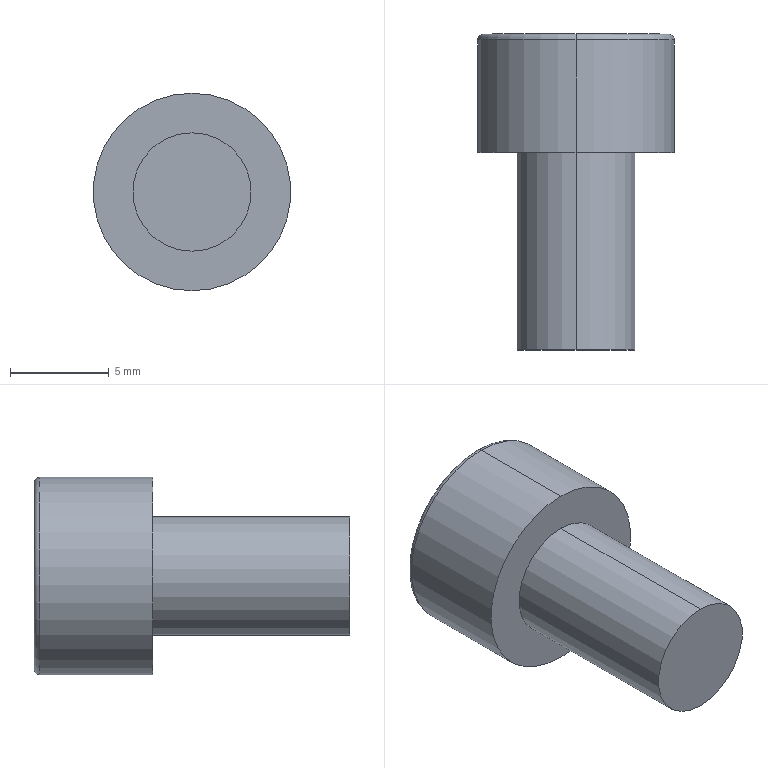Part | STEP file | M6 socket head cap screw simplified_M6X10 | 1 solid | 16 faces | box 10 x 16 x 10 mm | volume 685.808 mm3 | plane 10 | cylinder 4 | torus 2 | commonest cylinder face diameters 6 x2 10 x2
STEP:
#1=CARTESIAN_POINT('',(0.,0.,0.));
#2=DIRECTION('',(0.,0.,1.));
#3=DIRECTION('',(1.,0.,0.));
#4=AXIS2_PLACEMENT_3D('',#1,#2,#3);
#5=CARTESIAN_POINT('',(0.,0.,4.7));
#6=VERTEX_POINT('',#5);
#7=CARTESIAN_POINT('',(0.,0.,-4.7));
#8=VERTEX_POINT('',#7);
#9=CARTESIAN_POINT('',(0.,0.,0.));
#10=DIRECTION('',(0.,1.,0.));
#11=DIRECTION('',(0.,0.,-1.));
#12=AXIS2_PLACEMENT_3D('',#9,#10,#11);
#13=CIRCLE('',#12,4.7);
#14=CARTESIAN_POINT('',(0.,-0.3,0.));
#15=DIRECTION('',(0.,-1.,0.));
#16=DIRECTION('',(0.,0.,-1.));
#17=AXIS2_PLACEMENT_3D('',#14,#15,#16);
#18=TOROIDAL_SURFACE('',#17,4.7,0.3);
#19=CARTESIAN_POINT('',(6.283,4.712));
#20=DIRECTION('',(-1.,0.));
#21=VECTOR('',#20,1.);
#22=LINE('',#19,#21);
#23=(GEOMETRIC_REPRESENTATION_CONTEXT(2)PARAMETRIC_REPRESENTATION_CONTEXT()REPRESENTATION_CONTEXT('',''));
#24=DEFINITIONAL_REPRESENTATION('',(#22),#23);
#25=PCURVE('',#18,#24);
#26=CARTESIAN_POINT('',(0.,0.,0.));
#27=DIRECTION('',(0.,-1.,0.));
#28=DIRECTION('',(0.,0.,-1.));
#29=AXIS2_PLACEMENT_3D('',#26,#27,#28);
#30=PLANE('',#29);
#31=CARTESIAN_POINT('',(4.7,0.));
#32=CARTESIAN_POINT('',(4.7,-8.141));
#33=CARTESIAN_POINT('',(-2.35,-4.07));
#34=CARTESIAN_POINT('',(-9.4,0.));
#35=CARTESIAN_POINT('',(-2.35,4.07));
#36=CARTESIAN_POINT('',(4.7,8.141));
#37=CARTESIAN_POINT('',(4.7,0.));
#38=(BOUNDED_CURVE()B_SPLINE_CURVE(2,(#31,#32,#33,#34,#35,#36,#37),.UNSPECIFIED.,.T.,.F.)B_SPLINE_CURVE_WITH_KNOTS((1,2,2,2,2,1),(-2.094,0.,2.094,4.189,6.283,8.378),.UNSPECIFIED.)CURVE()GEOMETRIC_REPRESENTATION_ITEM()RATIONAL_B_SPLINE_CURVE((1.,0.5,1.,0.5,1.,0.5,1.))REPRESENTATION_ITEM(''));
#39=(GEOMETRIC_REPRESENTATION_CONTEXT(2)PARAMETRIC_REPRESENTATION_CONTEXT()REPRESENTATION_CONTEXT('',''));
#40=DEFINITIONAL_REPRESENTATION('',(#38),#39);
#41=PCURVE('',#30,#40);
#42=SURFACE_CURVE('',#13,(#25,#41),.PCURVE_S1.);
#43=EDGE_CURVE('',#6,#8,#42,.T.);
#44=ORIENTED_EDGE('',*,*,#43,.F.);
#45=CARTESIAN_POINT('',(0.,-0.3,5.));
#46=VERTEX_POINT('',#45);
#47=CARTESIAN_POINT('',(0.,-0.3,4.7));
#48=DIRECTION('',(1.,0.,0.));
#49=DIRECTION('',(0.,0.,-1.));
#50=AXIS2_PLACEMENT_3D('',#47,#48,#49);
#51=CIRCLE('',#50,0.3);
#52=CARTESIAN_POINT('',(3.142,3.142));
#53=DIRECTION('',(0.,1.));
#54=VECTOR('',#53,1.);
#55=LINE('',#52,#54);
#56=(GEOMETRIC_REPRESENTATION_CONTEXT(2)PARAMETRIC_REPRESENTATION_CONTEXT()REPRESENTATION_CONTEXT('',''));
#57=DEFINITIONAL_REPRESENTATION('',(#55),#56);
#58=PCURVE('',#18,#57);
#59=CARTESIAN_POINT('',(0.,-0.3,0.));
#60=DIRECTION('',(0.,-1.,0.));
#61=DIRECTION('',(0.,0.,-1.));
#62=AXIS2_PLACEMENT_3D('',#59,#60,#61);
#63=TOROIDAL_SURFACE('',#62,4.7,0.3);
#64=CARTESIAN_POINT('',(3.142,3.142));
#65=DIRECTION('',(0.,1.));
#66=VECTOR('',#65,1.);
#67=LINE('',#64,#66);
#68=(GEOMETRIC_REPRESENTATION_CONTEXT(2)PARAMETRIC_REPRESENTATION_CONTEXT()REPRESENTATION_CONTEXT('',''));
#69=DEFINITIONAL_REPRESENTATION('',(#67),#68);
#70=PCURVE('',#63,#69);
#71=SURFACE_CURVE('',#51,(#58,#70),.PCURVE_S1.);
#72=EDGE_CURVE('',#6,#46,#71,.T.);
#73=ORIENTED_EDGE('',*,*,#72,.T.);
#74=CARTESIAN_POINT('',(0.,-0.3,-5.));
#75=VERTEX_POINT('',#74);
#76=CARTESIAN_POINT('',(0.,-0.3,0.));
#77=DIRECTION('',(0.,-1.,0.));
#78=DIRECTION('',(0.,0.,-1.));
#79=AXIS2_PLACEMENT_3D('',#76,#77,#78);
#80=CIRCLE('',#79,5.);
#81=CARTESIAN_POINT('',(0.,6.283));
#82=DIRECTION('',(1.,0.));
#83=VECTOR('',#82,1.);
#84=LINE('',#81,#83);
#85=(GEOMETRIC_REPRESENTATION_CONTEXT(2)PARAMETRIC_REPRESENTATION_CONTEXT()REPRESENTATION_CONTEXT('',''));
#86=DEFINITIONAL_REPRESENTATION('',(#84),#85);
#87=PCURVE('',#18,#86);
#88=CARTESIAN_POINT('',(0.,0.,0.));
#89=DIRECTION('',(0.,1.,0.));
#90=DIRECTION('',(0.,0.,1.));
#91=AXIS2_PLACEMENT_3D('',#88,#89,#90);
#92=CYLINDRICAL_SURFACE('',#91,5.);
#93=CARTESIAN_POINT('',(3.142,-0.3));
#94=DIRECTION('',(-1.,0.));
#95=VECTOR('',#94,1.);
#96=LINE('',#93,#95);
#97=(GEOMETRIC_REPRESENTATION_CONTEXT(2)PARAMETRIC_REPRESENTATION_CONTEXT()REPRESENTATION_CONTEXT('',''));
#98=DEFINITIONAL_REPRESENTATION('',(#96),#97);
#99=PCURVE('',#92,#98);
#100=SURFACE_CURVE('',#80,(#87,#99),.PCURVE_S1.);
#101=EDGE_CURVE('',#75,#46,#100,.T.);
#102=ORIENTED_EDGE('',*,*,#101,.F.);
#103=CARTESIAN_POINT('',(0.,-0.3,-4.7));
#104=DIRECTION('',(-1.,0.,0.));
#105=DIRECTION('',(0.,0.,1.));
#106=AXIS2_PLACEMENT_3D('',#103,#104,#105);
#107=CIRCLE('',#106,0.3);
#108=CARTESIAN_POINT('',(0.,3.142));
#109=DIRECTION('',(0.,1.));
#110=VECTOR('',#109,1.);
#111=LINE('',#108,#110);
#112=(GEOMETRIC_REPRESENTATION_CONTEXT(2)PARAMETRIC_REPRESENTATION_CONTEXT()REPRESENTATION_CONTEXT('',''));
#113=DEFINITIONAL_REPRESENTATION('',(#111),#112);
#114=PCURVE('',#18,#113);
#115=CARTESIAN_POINT('',(6.283,3.142));
#116=DIRECTION('',(0.,1.));
#117=VECTOR('',#116,1.);
#118=LINE('',#115,#117);
#119=(GEOMETRIC_REPRESENTATION_CONTEXT(2)PARAMETRIC_REPRESENTATION_CONTEXT()REPRESENTATION_CONTEXT('',''));
#120=DEFINITIONAL_REPRESENTATION('',(#118),#119);
#121=PCURVE('',#63,#120);
#122=SURFACE_CURVE('',#107,(#114,#121),.PCURVE_S1.);
#123=EDGE_CURVE('',#8,#75,#122,.T.);
#124=ORIENTED_EDGE('',*,*,#123,.F.);
#125=EDGE_LOOP('',(#44,#73,#102,#124));
#126=FACE_BOUND('',#125,.T.);
#127=ADVANCED_FACE('',(#126),#18,.T.);
#128=CARTESIAN_POINT('',(0.,-16.,3.));
#129=VERTEX_POINT('',#128);
#130=CARTESIAN_POINT('',(0.,-16.,-3.));
#131=VERTEX_POINT('',#130);
#132=CARTESIAN_POINT('',(0.,-16.,0.));
#133=DIRECTION('',(0.,1.,0.));
#134=DIRECTION('',(0.,0.,1.));
#135=AXIS2_PLACEMENT_3D('',#132,#133,#134);
#136=CIRCLE('',#135,3.);
#137=CARTESIAN_POINT('',(0.,0.,0.));
#138=DIRECTION('',(0.,1.,0.));
#139=DIRECTION('',(0.,0.,1.));
#140=AXIS2_PLACEMENT_3D('',#137,#138,#139);
#141=CYLINDRICAL_SURFACE('',#140,3.);
#142=CARTESIAN_POINT('',(0.,-16.));
#143=DIRECTION('',(1.,0.));
#144=VECTOR('',#143,1.);
#145=LINE('',#142,#144);
#146=(GEOMETRIC_REPRESENTATION_CONTEXT(2)PARAMETRIC_REPRESENTATION_CONTEXT()REPRESENTATION_CONTEXT('',''));
#147=DEFINITIONAL_REPRESENTATION('',(#145),#146);
#148=PCURVE('',#141,#147);
#149=CARTESIAN_POINT('',(3.,-16.,0.));
#150=DIRECTION('',(0.,1.,0.));
#151=DIRECTION('',(0.,0.,1.));
#152=AXIS2_PLACEMENT_3D('',#149,#150,#151);
#153=PLANE('',#152);
#154=CARTESIAN_POINT('',(0.,-3.));
#155=DIRECTION('',(1.,0.));
#156=AXIS2_PLACEMENT_2D('',#154,#155);
#157=CIRCLE('',#156,3.);
#158=(GEOMETRIC_REPRESENTATION_CONTEXT(2)PARAMETRIC_REPRESENTATION_CONTEXT()REPRESENTATION_CONTEXT('',''));
#159=DEFINITIONAL_REPRESENTATION('',(#157),#158);
#160=PCURVE('',#153,#159);
#161=SURFACE_CURVE('',#136,(#148,#160),.PCURVE_S1.);
#162=EDGE_CURVE('',#129,#131,#161,.T.);
#163=ORIENTED_EDGE('',*,*,#162,.T.);
#164=CARTESIAN_POINT('',(0.,-6.,-3.));
#165=VERTEX_POINT('',#164);
#166=CARTESIAN_POINT('',(0.,0.,-3.));
#167=DIRECTION('',(0.,1.,0.));
#168=VECTOR('',#167,1.);
#169=LINE('',#166,#168);
#170=CARTESIAN_POINT('',(3.142,0.));
#171=DIRECTION('',(0.,1.));
#172=VECTOR('',#171,1.);
#173=LINE('',#170,#172);
#174=(GEOMETRIC_REPRESENTATION_CONTEXT(2)PARAMETRIC_REPRESENTATION_CONTEXT()REPRESENTATION_CONTEXT('',''));
#175=DEFINITIONAL_REPRESENTATION('',(#173),#174);
#176=PCURVE('',#141,#175);
#177=CARTESIAN_POINT('',(0.,0.,0.));
#178=DIRECTION('',(0.,1.,0.));
#179=DIRECTION('',(0.,0.,1.));
#180=AXIS2_PLACEMENT_3D('',#177,#178,#179);
#181=CYLINDRICAL_SURFACE('',#180,3.);
#182=CARTESIAN_POINT('',(3.142,0.));
#183=DIRECTION('',(0.,1.));
#184=VECTOR('',#183,1.);
#185=LINE('',#182,#184);
#186=(GEOMETRIC_REPRESENTATION_CONTEXT(2)PARAMETRIC_REPRESENTATION_CONTEXT()REPRESENTATION_CONTEXT('',''));
#187=DEFINITIONAL_REPRESENTATION('',(#185),#186);
#188=PCURVE('',#181,#187);
#189=SURFACE_CURVE('',#169,(#176,#188),.PCURVE_S1.);
#190=EDGE_CURVE('',#131,#165,#189,.T.);
#191=ORIENTED_EDGE('',*,*,#190,.T.);
#192=CARTESIAN_POINT('',(0.,-6.,3.));
#193=VERTEX_POINT('',#192);
#194=CARTESIAN_POINT('',(0.,-6.,0.));
#195=DIRECTION('',(0.,1.,0.));
#196=DIRECTION('',(0.,0.,1.));
#197=AXIS2_PLACEMENT_3D('',#194,#195,#196);
#198=CIRCLE('',#197,3.);
#199=CARTESIAN_POINT('',(0.,-6.));
#200=DIRECTION('',(1.,0.));
#201=VECTOR('',#200,1.);
#202=LINE('',#199,#201);
#203=(GEOMETRIC_REPRESENTATION_CONTEXT(2)PARAMETRIC_REPRESENTATION_CONTEXT()REPRESENTATION_CONTEXT('',''));
#204=DEFINITIONAL_REPRESENTATION('',(#202),#203);
#205=PCURVE('',#141,#204);
#206=CARTESIAN_POINT('',(5.,-6.,0.));
#207=DIRECTION('',(0.,1.,0.));
#208=DIRECTION('',(0.,0.,1.));
#209=AXIS2_PLACEMENT_3D('',#206,#207,#208);
#210=PLANE('',#209);
#211=CARTESIAN_POINT('',(0.,-5.));
#212=DIRECTION('',(1.,0.));
#213=AXIS2_PLACEMENT_2D('',#211,#212);
#214=CIRCLE('',#213,3.);
#215=(GEOMETRIC_REPRESENTATION_CONTEXT(2)PARAMETRIC_REPRESENTATION_CONTEXT()REPRESENTATION_CONTEXT('',''));
#216=DEFINITIONAL_REPRESENTATION('',(#214),#215);
#217=PCURVE('',#210,#216);
#218=SURFACE_CURVE('',#198,(#205,#217),.PCURVE_S1.);
#219=EDGE_CURVE('',#193,#165,#218,.T.);
#220=ORIENTED_EDGE('',*,*,#219,.F.);
#221=CARTESIAN_POINT('',(0.,0.,3.));
#222=DIRECTION('',(0.,1.,0.));
#223=VECTOR('',#222,1.);
#224=LINE('',#221,#223);
#225=CARTESIAN_POINT('',(0.,0.));
#226=DIRECTION('',(0.,1.));
#227=VECTOR('',#226,1.);
#228=LINE('',#225,#227);
#229=(GEOMETRIC_REPRESENTATION_CONTEXT(2)PARAMETRIC_REPRESENTATION_CONTEXT()REPRESENTATION_CONTEXT('',''));
#230=DEFINITIONAL_REPRESENTATION('',(#228),#229);
#231=PCURVE('',#141,#230);
#232=CARTESIAN_POINT('',(6.283,0.));
#233=DIRECTION('',(0.,1.));
#234=VECTOR('',#233,1.);
#235=LINE('',#232,#234);
#236=(GEOMETRIC_REPRESENTATION_CONTEXT(2)PARAMETRIC_REPRESENTATION_CONTEXT()REPRESENTATION_CONTEXT('',''));
#237=DEFINITIONAL_REPRESENTATION('',(#235),#236);
#238=PCURVE('',#181,#237);
#239=SURFACE_CURVE('',#224,(#231,#238),.PCURVE_S1.);
#240=EDGE_CURVE('',#129,#193,#239,.T.);
#241=ORIENTED_EDGE('',*,*,#240,.F.);
#242=EDGE_LOOP('',(#163,#191,#220,#241));
#243=FACE_BOUND('',#242,.T.);
#244=ADVANCED_FACE('',(#243),#141,.T.);
#245=CARTESIAN_POINT('',(0.,-6.,5.));
#246=VERTEX_POINT('',#245);
#247=CARTESIAN_POINT('',(0.,-6.,-5.));
#248=VERTEX_POINT('',#247);
#249=CARTESIAN_POINT('',(0.,-6.,0.));
#250=DIRECTION('',(0.,1.,0.));
#251=DIRECTION('',(0.,0.,1.));
#252=AXIS2_PLACEMENT_3D('',#249,#250,#251);
#253=CIRCLE('',#252,5.);
#254=CARTESIAN_POINT('',(0.,-6.));
#255=DIRECTION('',(1.,0.));
#256=VECTOR('',#255,1.);
#257=LINE('',#254,#256);
#258=(GEOMETRIC_REPRESENTATION_CONTEXT(2)PARAMETRIC_REPRESENTATION_CONTEXT()REPRESENTATION_CONTEXT('',''));
#259=DEFINITIONAL_REPRESENTATION('',(#257),#258);
#260=PCURVE('',#92,#259);
#261=CARTESIAN_POINT('',(0.,-5.));
#262=DIRECTION('',(1.,0.));
#263=AXIS2_PLACEMENT_2D('',#261,#262);
#264=CIRCLE('',#263,5.);
#265=(GEOMETRIC_REPRESENTATION_CONTEXT(2)PARAMETRIC_REPRESENTATION_CONTEXT()REPRESENTATION_CONTEXT('',''));
#266=DEFINITIONAL_REPRESENTATION('',(#264),#265);
#267=PCURVE('',#210,#266);
#268=SURFACE_CURVE('',#253,(#260,#267),.PCURVE_S1.);
#269=EDGE_CURVE('',#246,#248,#268,.T.);
#270=ORIENTED_EDGE('',*,*,#269,.T.);
#271=CARTESIAN_POINT('',(0.,0.,-5.));
#272=DIRECTION('',(0.,1.,0.));
#273=VECTOR('',#272,1.);
#274=LINE('',#271,#273);
#275=CARTESIAN_POINT('',(3.142,0.));
#276=DIRECTION('',(0.,1.));
#277=VECTOR('',#276,1.);
#278=LINE('',#275,#277);
#279=(GEOMETRIC_REPRESENTATION_CONTEXT(2)PARAMETRIC_REPRESENTATION_CONTEXT()REPRESENTATION_CONTEXT('',''));
#280=DEFINITIONAL_REPRESENTATION('',(#278),#279);
#281=PCURVE('',#92,#280);
#282=CARTESIAN_POINT('',(0.,0.,0.));
#283=DIRECTION('',(0.,1.,0.));
#284=DIRECTION('',(0.,0.,1.));
#285=AXIS2_PLACEMENT_3D('',#282,#283,#284);
#286=CYLINDRICAL_SURFACE('',#285,5.);
#287=CARTESIAN_POINT('',(3.142,0.));
#288=DIRECTION('',(0.,1.));
#289=VECTOR('',#288,1.);
#290=LINE('',#287,#289);
#291=(GEOMETRIC_REPRESENTATION_CONTEXT(2)PARAMETRIC_REPRESENTATION_CONTEXT()REPRESENTATION_CONTEXT('',''));
#292=DEFINITIONAL_REPRESENTATION('',(#290),#291);
#293=PCURVE('',#286,#292);
#294=SURFACE_CURVE('',#274,(#281,#293),.PCURVE_S1.);
#295=EDGE_CURVE('',#248,#75,#294,.T.);
#296=ORIENTED_EDGE('',*,*,#295,.T.);
#297=ORIENTED_EDGE('',*,*,#101,.T.);
#298=CARTESIAN_POINT('',(0.,0.,5.));
#299=DIRECTION('',(0.,1.,0.));
#300=VECTOR('',#299,1.);
#301=LINE('',#298,#300);
#302=CARTESIAN_POINT('',(0.,0.));
#303=DIRECTION('',(0.,1.));
#304=VECTOR('',#303,1.);
#305=LINE('',#302,#304);
#306=(GEOMETRIC_REPRESENTATION_CONTEXT(2)PARAMETRIC_REPRESENTATION_CONTEXT()REPRESENTATION_CONTEXT('',''));
#307=DEFINITIONAL_REPRESENTATION('',(#305),#306);
#308=PCURVE('',#92,#307);
#309=CARTESIAN_POINT('',(6.283,0.));
#310=DIRECTION('',(0.,1.));
#311=VECTOR('',#310,1.);
#312=LINE('',#309,#311);
#313=(GEOMETRIC_REPRESENTATION_CONTEXT(2)PARAMETRIC_REPRESENTATION_CONTEXT()REPRESENTATION_CONTEXT('',''));
#314=DEFINITIONAL_REPRESENTATION('',(#312),#313);
#315=PCURVE('',#286,#314);
#316=SURFACE_CURVE('',#301,(#308,#315),.PCURVE_S1.);
#317=EDGE_CURVE('',#246,#46,#316,.T.);
#318=ORIENTED_EDGE('',*,*,#317,.F.);
#319=EDGE_LOOP('',(#270,#296,#297,#318));
#320=FACE_BOUND('',#319,.T.);
#321=ADVANCED_FACE('',(#320),#92,.T.);
#322=CARTESIAN_POINT('',(0.,0.,0.));
#323=DIRECTION('',(0.,1.,0.));
#324=DIRECTION('',(0.,0.,-1.));
#325=AXIS2_PLACEMENT_3D('',#322,#323,#324);
#326=CIRCLE('',#325,4.7);
#327=CARTESIAN_POINT('',(4.7,0.));
#328=CARTESIAN_POINT('',(4.7,-8.141));
#329=CARTESIAN_POINT('',(-2.35,-4.07));
#330=CARTESIAN_POINT('',(-9.4,0.));
#331=CARTESIAN_POINT('',(-2.35,4.07));
#332=CARTESIAN_POINT('',(4.7,8.141));
#333=CARTESIAN_POINT('',(4.7,0.));
#334=(BOUNDED_CURVE()B_SPLINE_CURVE(2,(#327,#328,#329,#330,#331,#332,#333),.UNSPECIFIED.,.T.,.F.)B_SPLINE_CURVE_WITH_KNOTS((1,2,2,2,2,1),(-2.094,0.,2.094,4.189,6.283,8.378),.UNSPECIFIED.)CURVE()GEOMETRIC_REPRESENTATION_ITEM()RATIONAL_B_SPLINE_CURVE((1.,0.5,1.,0.5,1.,0.5,1.))REPRESENTATION_ITEM(''));
#335=(GEOMETRIC_REPRESENTATION_CONTEXT(2)PARAMETRIC_REPRESENTATION_CONTEXT()REPRESENTATION_CONTEXT('',''));
#336=DEFINITIONAL_REPRESENTATION('',(#334),#335);
#337=PCURVE('',#30,#336);
#338=CARTESIAN_POINT('',(6.283,4.712));
#339=DIRECTION('',(-1.,0.));
#340=VECTOR('',#339,1.);
#341=LINE('',#338,#340);
#342=(GEOMETRIC_REPRESENTATION_CONTEXT(2)PARAMETRIC_REPRESENTATION_CONTEXT()REPRESENTATION_CONTEXT('',''));
#343=DEFINITIONAL_REPRESENTATION('',(#341),#342);
#344=PCURVE('',#63,#343);
#345=SURFACE_CURVE('',#326,(#337,#344),.PCURVE_S1.);
#346=EDGE_CURVE('',#8,#6,#345,.T.);
#347=ORIENTED_EDGE('',*,*,#346,.T.);
#348=ORIENTED_EDGE('',*,*,#43,.T.);
#349=EDGE_LOOP('',(#347,#348));
#350=FACE_BOUND('',#349,.T.);
#351=CARTESIAN_POINT('',(-2.944,0.,0.));
#352=VERTEX_POINT('',#351);
#353=CARTESIAN_POINT('',(-1.472,0.,2.55));
#354=VERTEX_POINT('',#353);
#355=CARTESIAN_POINT('',(-2.944,0.,0.));
#356=DIRECTION('',(0.5,0.,0.866));
#357=VECTOR('',#356,1.);
#358=LINE('',#355,#357);
#359=CARTESIAN_POINT('',(0.,-2.944));
#360=DIRECTION('',(-0.866,0.5));
#361=VECTOR('',#360,1.);
#362=LINE('',#359,#361);
#363=(GEOMETRIC_REPRESENTATION_CONTEXT(2)PARAMETRIC_REPRESENTATION_CONTEXT()REPRESENTATION_CONTEXT('',''));
#364=DEFINITIONAL_REPRESENTATION('',(#362),#363);
#365=PCURVE('',#30,#364);
#366=CARTESIAN_POINT('',(-2.944,-3.,0.));
#367=DIRECTION('',(-0.866,0.,0.5));
#368=DIRECTION('',(0.5,0.,0.866));
#369=AXIS2_PLACEMENT_3D('',#366,#367,#368);
#370=PLANE('',#369);
#371=CARTESIAN_POINT('',(0.,3.));
#372=DIRECTION('',(1.,0.));
#373=VECTOR('',#372,1.);
#374=LINE('',#371,#373);
#375=(GEOMETRIC_REPRESENTATION_CONTEXT(2)PARAMETRIC_REPRESENTATION_CONTEXT()REPRESENTATION_CONTEXT('',''));
#376=DEFINITIONAL_REPRESENTATION('',(#374),#375);
#377=PCURVE('',#370,#376);
#378=SURFACE_CURVE('',#358,(#365,#377),.PCURVE_S1.);
#379=EDGE_CURVE('',#352,#354,#378,.T.);
#380=ORIENTED_EDGE('',*,*,#379,.F.);
#381=CARTESIAN_POINT('',(-1.472,0.,-2.55));
#382=VERTEX_POINT('',#381);
#383=CARTESIAN_POINT('',(-1.472,0.,-2.55));
#384=DIRECTION('',(-0.5,0.,0.866));
#385=VECTOR('',#384,1.);
#386=LINE('',#383,#385);
#387=CARTESIAN_POINT('',(2.55,-1.472));
#388=DIRECTION('',(-0.866,-0.5));
#389=VECTOR('',#388,1.);
#390=LINE('',#387,#389);
#391=(GEOMETRIC_REPRESENTATION_CONTEXT(2)PARAMETRIC_REPRESENTATION_CONTEXT()REPRESENTATION_CONTEXT('',''));
#392=DEFINITIONAL_REPRESENTATION('',(#390),#391);
#393=PCURVE('',#30,#392);
#394=CARTESIAN_POINT('',(-1.472,-3.,-2.55));
#395=DIRECTION('',(-0.866,0.,-0.5));
#396=DIRECTION('',(-0.5,0.,0.866));
#397=AXIS2_PLACEMENT_3D('',#394,#395,#396);
#398=PLANE('',#397);
#399=CARTESIAN_POINT('',(0.,3.));
#400=DIRECTION('',(1.,0.));
#401=VECTOR('',#400,1.);
#402=LINE('',#399,#401);
#403=(GEOMETRIC_REPRESENTATION_CONTEXT(2)PARAMETRIC_REPRESENTATION_CONTEXT()REPRESENTATION_CONTEXT('',''));
#404=DEFINITIONAL_REPRESENTATION('',(#402),#403);
#405=PCURVE('',#398,#404);
#406=SURFACE_CURVE('',#386,(#393,#405),.PCURVE_S1.);
#407=EDGE_CURVE('',#382,#352,#406,.T.);
#408=ORIENTED_EDGE('',*,*,#407,.F.);
#409=CARTESIAN_POINT('',(1.472,0.,-2.55));
#410=VERTEX_POINT('',#409);
#411=CARTESIAN_POINT('',(1.472,0.,-2.55));
#412=DIRECTION('',(-1.,0.,0.));
#413=VECTOR('',#412,1.);
#414=LINE('',#411,#413);
#415=CARTESIAN_POINT('',(2.55,1.472));
#416=DIRECTION('',(0.,-1.));
#417=VECTOR('',#416,1.);
#418=LINE('',#415,#417);
#419=(GEOMETRIC_REPRESENTATION_CONTEXT(2)PARAMETRIC_REPRESENTATION_CONTEXT()REPRESENTATION_CONTEXT('',''));
#420=DEFINITIONAL_REPRESENTATION('',(#418),#419);
#421=PCURVE('',#30,#420);
#422=CARTESIAN_POINT('',(1.472,-3.,-2.55));
#423=DIRECTION('',(0.,0.,-1.));
#424=DIRECTION('',(-1.,0.,0.));
#425=AXIS2_PLACEMENT_3D('',#422,#423,#424);
#426=PLANE('',#425);
#427=CARTESIAN_POINT('',(0.,3.));
#428=DIRECTION('',(1.,0.));
#429=VECTOR('',#428,1.);
#430=LINE('',#427,#429);
#431=(GEOMETRIC_REPRESENTATION_CONTEXT(2)PARAMETRIC_REPRESENTATION_CONTEXT()REPRESENTATION_CONTEXT('',''));
#432=DEFINITIONAL_REPRESENTATION('',(#430),#431);
#433=PCURVE('',#426,#432);
#434=SURFACE_CURVE('',#414,(#421,#433),.PCURVE_S1.);
#435=EDGE_CURVE('',#410,#382,#434,.T.);
#436=ORIENTED_EDGE('',*,*,#435,.F.);
#437=CARTESIAN_POINT('',(2.944,0.,0.));
#438=VERTEX_POINT('',#437);
#439=CARTESIAN_POINT('',(2.944,0.,0.));
#440=DIRECTION('',(-0.5,0.,-0.866));
#441=VECTOR('',#440,1.);
#442=LINE('',#439,#441);
#443=CARTESIAN_POINT('',(0.,2.944));
#444=DIRECTION('',(0.866,-0.5));
#445=VECTOR('',#444,1.);
#446=LINE('',#443,#445);
#447=(GEOMETRIC_REPRESENTATION_CONTEXT(2)PARAMETRIC_REPRESENTATION_CONTEXT()REPRESENTATION_CONTEXT('',''));
#448=DEFINITIONAL_REPRESENTATION('',(#446),#447);
#449=PCURVE('',#30,#448);
#450=CARTESIAN_POINT('',(2.944,-3.,0.));
#451=DIRECTION('',(0.866,0.,-0.5));
#452=DIRECTION('',(-0.5,0.,-0.866));
#453=AXIS2_PLACEMENT_3D('',#450,#451,#452);
#454=PLANE('',#453);
#455=CARTESIAN_POINT('',(0.,3.));
#456=DIRECTION('',(1.,0.));
#457=VECTOR('',#456,1.);
#458=LINE('',#455,#457);
#459=(GEOMETRIC_REPRESENTATION_CONTEXT(2)PARAMETRIC_REPRESENTATION_CONTEXT()REPRESENTATION_CONTEXT('',''));
#460=DEFINITIONAL_REPRESENTATION('',(#458),#459);
#461=PCURVE('',#454,#460);
#462=SURFACE_CURVE('',#442,(#449,#461),.PCURVE_S1.);
#463=EDGE_CURVE('',#438,#410,#462,.T.);
#464=ORIENTED_EDGE('',*,*,#463,.F.);
#465=CARTESIAN_POINT('',(1.472,0.,2.55));
#466=VERTEX_POINT('',#465);
#467=CARTESIAN_POINT('',(1.472,0.,2.55));
#468=DIRECTION('',(0.5,0.,-0.866));
#469=VECTOR('',#468,1.);
#470=LINE('',#467,#469);
#471=CARTESIAN_POINT('',(-2.55,1.472));
#472=DIRECTION('',(0.866,0.5));
#473=VECTOR('',#472,1.);
#474=LINE('',#471,#473);
#475=(GEOMETRIC_REPRESENTATION_CONTEXT(2)PARAMETRIC_REPRESENTATION_CONTEXT()REPRESENTATION_CONTEXT('',''));
#476=DEFINITIONAL_REPRESENTATION('',(#474),#475);
#477=PCURVE('',#30,#476);
#478=CARTESIAN_POINT('',(1.472,-3.,2.55));
#479=DIRECTION('',(0.866,0.,0.5));
#480=DIRECTION('',(0.5,0.,-0.866));
#481=AXIS2_PLACEMENT_3D('',#478,#479,#480);
#482=PLANE('',#481);
#483=CARTESIAN_POINT('',(0.,3.));
#484=DIRECTION('',(1.,0.));
#485=VECTOR('',#484,1.);
#486=LINE('',#483,#485);
#487=(GEOMETRIC_REPRESENTATION_CONTEXT(2)PARAMETRIC_REPRESENTATION_CONTEXT()REPRESENTATION_CONTEXT('',''));
#488=DEFINITIONAL_REPRESENTATION('',(#486),#487);
#489=PCURVE('',#482,#488);
#490=SURFACE_CURVE('',#470,(#477,#489),.PCURVE_S1.);
#491=EDGE_CURVE('',#466,#438,#490,.T.);
#492=ORIENTED_EDGE('',*,*,#491,.F.);
#493=CARTESIAN_POINT('',(-1.472,0.,2.55));
#494=DIRECTION('',(1.,0.,0.));
#495=VECTOR('',#494,1.);
#496=LINE('',#493,#495);
#497=CARTESIAN_POINT('',(-2.55,-1.472));
#498=DIRECTION('',(0.,1.));
#499=VECTOR('',#498,1.);
#500=LINE('',#497,#499);
#501=(GEOMETRIC_REPRESENTATION_CONTEXT(2)PARAMETRIC_REPRESENTATION_CONTEXT()REPRESENTATION_CONTEXT('',''));
#502=DEFINITIONAL_REPRESENTATION('',(#500),#501);
#503=PCURVE('',#30,#502);
#504=CARTESIAN_POINT('',(-1.472,-3.,2.55));
#505=DIRECTION('',(0.,0.,1.));
#506=DIRECTION('',(1.,0.,0.));
#507=AXIS2_PLACEMENT_3D('',#504,#505,#506);
#508=PLANE('',#507);
#509=CARTESIAN_POINT('',(0.,3.));
#510=DIRECTION('',(1.,0.));
#511=VECTOR('',#510,1.);
#512=LINE('',#509,#511);
#513=(GEOMETRIC_REPRESENTATION_CONTEXT(2)PARAMETRIC_REPRESENTATION_CONTEXT()REPRESENTATION_CONTEXT('',''));
#514=DEFINITIONAL_REPRESENTATION('',(#512),#513);
#515=PCURVE('',#508,#514);
#516=SURFACE_CURVE('',#496,(#503,#515),.PCURVE_S1.);
#517=EDGE_CURVE('',#354,#466,#516,.T.);
#518=ORIENTED_EDGE('',*,*,#517,.F.);
#519=EDGE_LOOP('',(#380,#408,#436,#464,#492,#518));
#520=FACE_BOUND('',#519,.T.);
#521=ADVANCED_FACE('',(#350,#520),#30,.F.);
#522=ORIENTED_EDGE('',*,*,#295,.F.);
#523=CARTESIAN_POINT('',(0.,-6.,0.));
#524=DIRECTION('',(0.,1.,0.));
#525=DIRECTION('',(0.,0.,1.));
#526=AXIS2_PLACEMENT_3D('',#523,#524,#525);
#527=CIRCLE('',#526,5.);
#528=CARTESIAN_POINT('',(0.,-6.));
#529=DIRECTION('',(1.,0.));
#530=VECTOR('',#529,1.);
#531=LINE('',#528,#530);
#532=(GEOMETRIC_REPRESENTATION_CONTEXT(2)PARAMETRIC_REPRESENTATION_CONTEXT()REPRESENTATION_CONTEXT('',''));
#533=DEFINITIONAL_REPRESENTATION('',(#531),#532);
#534=PCURVE('',#286,#533);
#535=CARTESIAN_POINT('',(0.,-5.));
#536=DIRECTION('',(1.,0.));
#537=AXIS2_PLACEMENT_2D('',#535,#536);
#538=CIRCLE('',#537,5.);
#539=(GEOMETRIC_REPRESENTATION_CONTEXT(2)PARAMETRIC_REPRESENTATION_CONTEXT()REPRESENTATION_CONTEXT('',''));
#540=DEFINITIONAL_REPRESENTATION('',(#538),#539);
#541=PCURVE('',#210,#540);
#542=SURFACE_CURVE('',#527,(#534,#541),.PCURVE_S1.);
#543=EDGE_CURVE('',#248,#246,#542,.T.);
#544=ORIENTED_EDGE('',*,*,#543,.T.);
#545=ORIENTED_EDGE('',*,*,#317,.T.);
#546=CARTESIAN_POINT('',(0.,-0.3,0.));
#547=DIRECTION('',(0.,-1.,0.));
#548=DIRECTION('',(0.,0.,-1.));
#549=AXIS2_PLACEMENT_3D('',#546,#547,#548);
#550=CIRCLE('',#549,5.);
#551=CARTESIAN_POINT('',(9.425,-0.3));
#552=DIRECTION('',(-1.,0.));
#553=VECTOR('',#552,1.);
#554=LINE('',#551,#553);
#555=(GEOMETRIC_REPRESENTATION_CONTEXT(2)PARAMETRIC_REPRESENTATION_CONTEXT()REPRESENTATION_CONTEXT('',''));
#556=DEFINITIONAL_REPRESENTATION('',(#554),#555);
#557=PCURVE('',#286,#556);
#558=CARTESIAN_POINT('',(0.,6.283));
#559=DIRECTION('',(1.,0.));
#560=VECTOR('',#559,1.);
#561=LINE('',#558,#560);
#562=(GEOMETRIC_REPRESENTATION_CONTEXT(2)PARAMETRIC_REPRESENTATION_CONTEXT()REPRESENTATION_CONTEXT('',''));
#563=DEFINITIONAL_REPRESENTATION('',(#561),#562);
#564=PCURVE('',#63,#563);
#565=SURFACE_CURVE('',#550,(#557,#564),.PCURVE_S1.);
#566=EDGE_CURVE('',#46,#75,#565,.T.);
#567=ORIENTED_EDGE('',*,*,#566,.T.);
#568=EDGE_LOOP('',(#522,#544,#545,#567));
#569=FACE_BOUND('',#568,.T.);
#570=ADVANCED_FACE('',(#569),#286,.T.);
#571=ORIENTED_EDGE('',*,*,#269,.F.);
#572=ORIENTED_EDGE('',*,*,#543,.F.);
#573=EDGE_LOOP('',(#571,#572));
#574=FACE_BOUND('',#573,.T.);
#575=ORIENTED_EDGE('',*,*,#219,.T.);
#576=CARTESIAN_POINT('',(0.,-6.,0.));
#577=DIRECTION('',(0.,1.,0.));
#578=DIRECTION('',(0.,0.,1.));
#579=AXIS2_PLACEMENT_3D('',#576,#577,#578);
#580=CIRCLE('',#579,3.);
#581=CARTESIAN_POINT('',(0.,-5.));
#582=DIRECTION('',(1.,0.));
#583=AXIS2_PLACEMENT_2D('',#581,#582);
#584=CIRCLE('',#583,3.);
#585=(GEOMETRIC_REPRESENTATION_CONTEXT(2)PARAMETRIC_REPRESENTATION_CONTEXT()REPRESENTATION_CONTEXT('',''));
#586=DEFINITIONAL_REPRESENTATION('',(#584),#585);
#587=PCURVE('',#210,#586);
#588=CARTESIAN_POINT('',(0.,-6.));
#589=DIRECTION('',(1.,0.));
#590=VECTOR('',#589,1.);
#591=LINE('',#588,#590);
#592=(GEOMETRIC_REPRESENTATION_CONTEXT(2)PARAMETRIC_REPRESENTATION_CONTEXT()REPRESENTATION_CONTEXT('',''));
#593=DEFINITIONAL_REPRESENTATION('',(#591),#592);
#594=PCURVE('',#181,#593);
#595=SURFACE_CURVE('',#580,(#587,#594),.PCURVE_S1.);
#596=EDGE_CURVE('',#165,#193,#595,.T.);
#597=ORIENTED_EDGE('',*,*,#596,.T.);
#598=EDGE_LOOP('',(#575,#597));
#599=FACE_BOUND('',#598,.T.);
#600=ADVANCED_FACE('',(#574,#599),#210,.F.);
#601=ORIENTED_EDGE('',*,*,#190,.F.);
#602=CARTESIAN_POINT('',(0.,-16.,0.));
#603=DIRECTION('',(0.,1.,0.));
#604=DIRECTION('',(0.,0.,1.));
#605=AXIS2_PLACEMENT_3D('',#602,#603,#604);
#606=CIRCLE('',#605,3.);
#607=CARTESIAN_POINT('',(0.,-16.));
#608=DIRECTION('',(1.,0.));
#609=VECTOR('',#608,1.);
#610=LINE('',#607,#609);
#611=(GEOMETRIC_REPRESENTATION_CONTEXT(2)PARAMETRIC_REPRESENTATION_CONTEXT()REPRESENTATION_CONTEXT('',''));
#612=DEFINITIONAL_REPRESENTATION('',(#610),#611);
#613=PCURVE('',#181,#612);
#614=CARTESIAN_POINT('',(0.,-3.));
#615=DIRECTION('',(1.,0.));
#616=AXIS2_PLACEMENT_2D('',#614,#615);
#617=CIRCLE('',#616,3.);
#618=(GEOMETRIC_REPRESENTATION_CONTEXT(2)PARAMETRIC_REPRESENTATION_CONTEXT()REPRESENTATION_CONTEXT('',''));
#619=DEFINITIONAL_REPRESENTATION('',(#617),#618);
#620=PCURVE('',#153,#619);
#621=SURFACE_CURVE('',#606,(#613,#620),.PCURVE_S1.);
#622=EDGE_CURVE('',#131,#129,#621,.T.);
#623=ORIENTED_EDGE('',*,*,#622,.T.);
#624=ORIENTED_EDGE('',*,*,#240,.T.);
#625=ORIENTED_EDGE('',*,*,#596,.F.);
#626=EDGE_LOOP('',(#601,#623,#624,#625));
#627=FACE_BOUND('',#626,.T.);
#628=ADVANCED_FACE('',(#627),#181,.T.);
#629=ORIENTED_EDGE('',*,*,#162,.F.);
#630=ORIENTED_EDGE('',*,*,#622,.F.);
#631=EDGE_LOOP('',(#629,#630));
#632=FACE_BOUND('',#631,.T.);
#633=ADVANCED_FACE('',(#632),#153,.F.);
#634=ORIENTED_EDGE('',*,*,#407,.T.);
#635=CARTESIAN_POINT('',(-2.944,-3.,0.));
#636=VERTEX_POINT('',#635);
#637=CARTESIAN_POINT('',(-2.944,-3.,0.));
#638=DIRECTION('',(0.,1.,0.));
#639=VECTOR('',#638,1.);
#640=LINE('',#637,#639);
#641=CARTESIAN_POINT('',(2.944,0.));
#642=DIRECTION('',(0.,1.));
#643=VECTOR('',#642,1.);
#644=LINE('',#641,#643);
#645=(GEOMETRIC_REPRESENTATION_CONTEXT(2)PARAMETRIC_REPRESENTATION_CONTEXT()REPRESENTATION_CONTEXT('',''));
#646=DEFINITIONAL_REPRESENTATION('',(#644),#645);
#647=PCURVE('',#398,#646);
#648=CARTESIAN_POINT('',(0.,0.));
#649=DIRECTION('',(0.,1.));
#650=VECTOR('',#649,1.);
#651=LINE('',#648,#650);
#652=(GEOMETRIC_REPRESENTATION_CONTEXT(2)PARAMETRIC_REPRESENTATION_CONTEXT()REPRESENTATION_CONTEXT('',''));
#653=DEFINITIONAL_REPRESENTATION('',(#651),#652);
#654=PCURVE('',#370,#653);
#655=SURFACE_CURVE('',#640,(#647,#654),.PCURVE_S1.);
#656=EDGE_CURVE('',#636,#352,#655,.T.);
#657=ORIENTED_EDGE('',*,*,#656,.F.);
#658=CARTESIAN_POINT('',(-1.472,-3.,-2.55));
#659=VERTEX_POINT('',#658);
#660=CARTESIAN_POINT('',(-1.472,-3.,-2.55));
#661=DIRECTION('',(-0.5,0.,0.866));
#662=VECTOR('',#661,1.);
#663=LINE('',#660,#662);
#664=CARTESIAN_POINT('',(0.,0.));
#665=DIRECTION('',(1.,0.));
#666=VECTOR('',#665,1.);
#667=LINE('',#664,#666);
#668=(GEOMETRIC_REPRESENTATION_CONTEXT(2)PARAMETRIC_REPRESENTATION_CONTEXT()REPRESENTATION_CONTEXT('',''));
#669=DEFINITIONAL_REPRESENTATION('',(#667),#668);
#670=PCURVE('',#398,#669);
#671=CARTESIAN_POINT('',(-2.944,-3.,0.));
#672=DIRECTION('',(0.,1.,0.));
#673=DIRECTION('',(0.,0.,1.));
#674=AXIS2_PLACEMENT_3D('',#671,#672,#673);
#675=PLANE('',#674);
#676=CARTESIAN_POINT('',(-2.55,1.472));
#677=DIRECTION('',(0.866,-0.5));
#678=VECTOR('',#677,1.);
#679=LINE('',#676,#678);
#680=(GEOMETRIC_REPRESENTATION_CONTEXT(2)PARAMETRIC_REPRESENTATION_CONTEXT()REPRESENTATION_CONTEXT('',''));
#681=DEFINITIONAL_REPRESENTATION('',(#679),#680);
#682=PCURVE('',#675,#681);
#683=SURFACE_CURVE('',#663,(#670,#682),.PCURVE_S1.);
#684=EDGE_CURVE('',#659,#636,#683,.T.);
#685=ORIENTED_EDGE('',*,*,#684,.F.);
#686=CARTESIAN_POINT('',(-1.472,-3.,-2.55));
#687=DIRECTION('',(0.,1.,0.));
#688=VECTOR('',#687,1.);
#689=LINE('',#686,#688);
#690=CARTESIAN_POINT('',(0.,0.));
#691=DIRECTION('',(0.,1.));
#692=VECTOR('',#691,1.);
#693=LINE('',#690,#692);
#694=(GEOMETRIC_REPRESENTATION_CONTEXT(2)PARAMETRIC_REPRESENTATION_CONTEXT()REPRESENTATION_CONTEXT('',''));
#695=DEFINITIONAL_REPRESENTATION('',(#693),#694);
#696=PCURVE('',#398,#695);
#697=CARTESIAN_POINT('',(2.944,0.));
#698=DIRECTION('',(0.,1.));
#699=VECTOR('',#698,1.);
#700=LINE('',#697,#699);
#701=(GEOMETRIC_REPRESENTATION_CONTEXT(2)PARAMETRIC_REPRESENTATION_CONTEXT()REPRESENTATION_CONTEXT('',''));
#702=DEFINITIONAL_REPRESENTATION('',(#700),#701);
#703=PCURVE('',#426,#702);
#704=SURFACE_CURVE('',#689,(#696,#703),.PCURVE_S1.);
#705=EDGE_CURVE('',#659,#382,#704,.T.);
#706=ORIENTED_EDGE('',*,*,#705,.T.);
#707=EDGE_LOOP('',(#634,#657,#685,#706));
#708=FACE_BOUND('',#707,.T.);
#709=ADVANCED_FACE('',(#708),#398,.F.);
#710=ORIENTED_EDGE('',*,*,#435,.T.);
#711=ORIENTED_EDGE('',*,*,#705,.F.);
#712=CARTESIAN_POINT('',(1.472,-3.,-2.55));
#713=VERTEX_POINT('',#712);
#714=CARTESIAN_POINT('',(1.472,-3.,-2.55));
#715=DIRECTION('',(-1.,0.,0.));
#716=VECTOR('',#715,1.);
#717=LINE('',#714,#716);
#718=CARTESIAN_POINT('',(0.,0.));
#719=DIRECTION('',(1.,0.));
#720=VECTOR('',#719,1.);
#721=LINE('',#718,#720);
#722=(GEOMETRIC_REPRESENTATION_CONTEXT(2)PARAMETRIC_REPRESENTATION_CONTEXT()REPRESENTATION_CONTEXT('',''));
#723=DEFINITIONAL_REPRESENTATION('',(#721),#722);
#724=PCURVE('',#426,#723);
#725=CARTESIAN_POINT('',(-2.55,4.417));
#726=DIRECTION('',(0.,-1.));
#727=VECTOR('',#726,1.);
#728=LINE('',#725,#727);
#729=(GEOMETRIC_REPRESENTATION_CONTEXT(2)PARAMETRIC_REPRESENTATION_CONTEXT()REPRESENTATION_CONTEXT('',''));
#730=DEFINITIONAL_REPRESENTATION('',(#728),#729);
#731=PCURVE('',#675,#730);
#732=SURFACE_CURVE('',#717,(#724,#731),.PCURVE_S1.);
#733=EDGE_CURVE('',#713,#659,#732,.T.);
#734=ORIENTED_EDGE('',*,*,#733,.F.);
#735=CARTESIAN_POINT('',(1.472,-3.,-2.55));
#736=DIRECTION('',(0.,1.,0.));
#737=VECTOR('',#736,1.);
#738=LINE('',#735,#737);
#739=CARTESIAN_POINT('',(0.,0.));
#740=DIRECTION('',(0.,1.));
#741=VECTOR('',#740,1.);
#742=LINE('',#739,#741);
#743=(GEOMETRIC_REPRESENTATION_CONTEXT(2)PARAMETRIC_REPRESENTATION_CONTEXT()REPRESENTATION_CONTEXT('',''));
#744=DEFINITIONAL_REPRESENTATION('',(#742),#743);
#745=PCURVE('',#426,#744);
#746=CARTESIAN_POINT('',(2.944,0.));
#747=DIRECTION('',(0.,1.));
#748=VECTOR('',#747,1.);
#749=LINE('',#746,#748);
#750=(GEOMETRIC_REPRESENTATION_CONTEXT(2)PARAMETRIC_REPRESENTATION_CONTEXT()REPRESENTATION_CONTEXT('',''));
#751=DEFINITIONAL_REPRESENTATION('',(#749),#750);
#752=PCURVE('',#454,#751);
#753=SURFACE_CURVE('',#738,(#745,#752),.PCURVE_S1.);
#754=EDGE_CURVE('',#713,#410,#753,.T.);
#755=ORIENTED_EDGE('',*,*,#754,.T.);
#756=EDGE_LOOP('',(#710,#711,#734,#755));
#757=FACE_BOUND('',#756,.T.);
#758=ADVANCED_FACE('',(#757),#426,.F.);
#759=ORIENTED_EDGE('',*,*,#463,.T.);
#760=ORIENTED_EDGE('',*,*,#754,.F.);
#761=CARTESIAN_POINT('',(2.944,-3.,0.));
#762=VERTEX_POINT('',#761);
#763=CARTESIAN_POINT('',(2.944,-3.,0.));
#764=DIRECTION('',(-0.5,0.,-0.866));
#765=VECTOR('',#764,1.);
#766=LINE('',#763,#765);
#767=CARTESIAN_POINT('',(0.,0.));
#768=DIRECTION('',(1.,0.));
#769=VECTOR('',#768,1.);
#770=LINE('',#767,#769);
#771=(GEOMETRIC_REPRESENTATION_CONTEXT(2)PARAMETRIC_REPRESENTATION_CONTEXT()REPRESENTATION_CONTEXT('',''));
#772=DEFINITIONAL_REPRESENTATION('',(#770),#771);
#773=PCURVE('',#454,#772);
#774=CARTESIAN_POINT('',(0.,5.889));
#775=DIRECTION('',(-0.866,-0.5));
#776=VECTOR('',#775,1.);
#777=LINE('',#774,#776);
#778=(GEOMETRIC_REPRESENTATION_CONTEXT(2)PARAMETRIC_REPRESENTATION_CONTEXT()REPRESENTATION_CONTEXT('',''));
#779=DEFINITIONAL_REPRESENTATION('',(#777),#778);
#780=PCURVE('',#675,#779);
#781=SURFACE_CURVE('',#766,(#773,#780),.PCURVE_S1.);
#782=EDGE_CURVE('',#762,#713,#781,.T.);
#783=ORIENTED_EDGE('',*,*,#782,.F.);
#784=CARTESIAN_POINT('',(2.944,-3.,0.));
#785=DIRECTION('',(0.,1.,0.));
#786=VECTOR('',#785,1.);
#787=LINE('',#784,#786);
#788=CARTESIAN_POINT('',(0.,0.));
#789=DIRECTION('',(0.,1.));
#790=VECTOR('',#789,1.);
#791=LINE('',#788,#790);
#792=(GEOMETRIC_REPRESENTATION_CONTEXT(2)PARAMETRIC_REPRESENTATION_CONTEXT()REPRESENTATION_CONTEXT('',''));
#793=DEFINITIONAL_REPRESENTATION('',(#791),#792);
#794=PCURVE('',#454,#793);
#795=CARTESIAN_POINT('',(2.944,0.));
#796=DIRECTION('',(0.,1.));
#797=VECTOR('',#796,1.);
#798=LINE('',#795,#797);
#799=(GEOMETRIC_REPRESENTATION_CONTEXT(2)PARAMETRIC_REPRESENTATION_CONTEXT()REPRESENTATION_CONTEXT('',''));
#800=DEFINITIONAL_REPRESENTATION('',(#798),#799);
#801=PCURVE('',#482,#800);
#802=SURFACE_CURVE('',#787,(#794,#801),.PCURVE_S1.);
#803=EDGE_CURVE('',#762,#438,#802,.T.);
#804=ORIENTED_EDGE('',*,*,#803,.T.);
#805=EDGE_LOOP('',(#759,#760,#783,#804));
#806=FACE_BOUND('',#805,.T.);
#807=ADVANCED_FACE('',(#806),#454,.F.);
#808=ORIENTED_EDGE('',*,*,#491,.T.);
#809=ORIENTED_EDGE('',*,*,#803,.F.);
#810=CARTESIAN_POINT('',(1.472,-3.,2.55));
#811=VERTEX_POINT('',#810);
#812=CARTESIAN_POINT('',(1.472,-3.,2.55));
#813=DIRECTION('',(0.5,0.,-0.866));
#814=VECTOR('',#813,1.);
#815=LINE('',#812,#814);
#816=CARTESIAN_POINT('',(0.,0.));
#817=DIRECTION('',(1.,0.));
#818=VECTOR('',#817,1.);
#819=LINE('',#816,#818);
#820=(GEOMETRIC_REPRESENTATION_CONTEXT(2)PARAMETRIC_REPRESENTATION_CONTEXT()REPRESENTATION_CONTEXT('',''));
#821=DEFINITIONAL_REPRESENTATION('',(#819),#820);
#822=PCURVE('',#482,#821);
#823=CARTESIAN_POINT('',(2.55,4.417));
#824=DIRECTION('',(-0.866,0.5));
#825=VECTOR('',#824,1.);
#826=LINE('',#823,#825);
#827=(GEOMETRIC_REPRESENTATION_CONTEXT(2)PARAMETRIC_REPRESENTATION_CONTEXT()REPRESENTATION_CONTEXT('',''));
#828=DEFINITIONAL_REPRESENTATION('',(#826),#827);
#829=PCURVE('',#675,#828);
#830=SURFACE_CURVE('',#815,(#822,#829),.PCURVE_S1.);
#831=EDGE_CURVE('',#811,#762,#830,.T.);
#832=ORIENTED_EDGE('',*,*,#831,.F.);
#833=CARTESIAN_POINT('',(1.472,-3.,2.55));
#834=DIRECTION('',(0.,1.,0.));
#835=VECTOR('',#834,1.);
#836=LINE('',#833,#835);
#837=CARTESIAN_POINT('',(0.,0.));
#838=DIRECTION('',(0.,1.));
#839=VECTOR('',#838,1.);
#840=LINE('',#837,#839);
#841=(GEOMETRIC_REPRESENTATION_CONTEXT(2)PARAMETRIC_REPRESENTATION_CONTEXT()REPRESENTATION_CONTEXT('',''));
#842=DEFINITIONAL_REPRESENTATION('',(#840),#841);
#843=PCURVE('',#482,#842);
#844=CARTESIAN_POINT('',(2.944,0.));
#845=DIRECTION('',(0.,1.));
#846=VECTOR('',#845,1.);
#847=LINE('',#844,#846);
#848=(GEOMETRIC_REPRESENTATION_CONTEXT(2)PARAMETRIC_REPRESENTATION_CONTEXT()REPRESENTATION_CONTEXT('',''));
#849=DEFINITIONAL_REPRESENTATION('',(#847),#848);
#850=PCURVE('',#508,#849);
#851=SURFACE_CURVE('',#836,(#843,#850),.PCURVE_S1.);
#852=EDGE_CURVE('',#811,#466,#851,.T.);
#853=ORIENTED_EDGE('',*,*,#852,.T.);
#854=EDGE_LOOP('',(#808,#809,#832,#853));
#855=FACE_BOUND('',#854,.T.);
#856=ADVANCED_FACE('',(#855),#482,.F.);
#857=ORIENTED_EDGE('',*,*,#517,.T.);
#858=ORIENTED_EDGE('',*,*,#852,.F.);
#859=CARTESIAN_POINT('',(-1.472,-3.,2.55));
#860=VERTEX_POINT('',#859);
#861=CARTESIAN_POINT('',(-1.472,-3.,2.55));
#862=DIRECTION('',(1.,0.,0.));
#863=VECTOR('',#862,1.);
#864=LINE('',#861,#863);
#865=CARTESIAN_POINT('',(0.,0.));
#866=DIRECTION('',(1.,0.));
#867=VECTOR('',#866,1.);
#868=LINE('',#865,#867);
#869=(GEOMETRIC_REPRESENTATION_CONTEXT(2)PARAMETRIC_REPRESENTATION_CONTEXT()REPRESENTATION_CONTEXT('',''));
#870=DEFINITIONAL_REPRESENTATION('',(#868),#869);
#871=PCURVE('',#508,#870);
#872=CARTESIAN_POINT('',(2.55,1.472));
#873=DIRECTION('',(0.,1.));
#874=VECTOR('',#873,1.);
#875=LINE('',#872,#874);
#876=(GEOMETRIC_REPRESENTATION_CONTEXT(2)PARAMETRIC_REPRESENTATION_CONTEXT()REPRESENTATION_CONTEXT('',''));
#877=DEFINITIONAL_REPRESENTATION('',(#875),#876);
#878=PCURVE('',#675,#877);
#879=SURFACE_CURVE('',#864,(#871,#878),.PCURVE_S1.);
#880=EDGE_CURVE('',#860,#811,#879,.T.);
#881=ORIENTED_EDGE('',*,*,#880,.F.);
#882=CARTESIAN_POINT('',(-1.472,-3.,2.55));
#883=DIRECTION('',(0.,1.,0.));
#884=VECTOR('',#883,1.);
#885=LINE('',#882,#884);
#886=CARTESIAN_POINT('',(0.,0.));
#887=DIRECTION('',(0.,1.));
#888=VECTOR('',#887,1.);
#889=LINE('',#886,#888);
#890=(GEOMETRIC_REPRESENTATION_CONTEXT(2)PARAMETRIC_REPRESENTATION_CONTEXT()REPRESENTATION_CONTEXT('',''));
#891=DEFINITIONAL_REPRESENTATION('',(#889),#890);
#892=PCURVE('',#508,#891);
#893=CARTESIAN_POINT('',(2.944,0.));
#894=DIRECTION('',(0.,1.));
#895=VECTOR('',#894,1.);
#896=LINE('',#893,#895);
#897=(GEOMETRIC_REPRESENTATION_CONTEXT(2)PARAMETRIC_REPRESENTATION_CONTEXT()REPRESENTATION_CONTEXT('',''));
#898=DEFINITIONAL_REPRESENTATION('',(#896),#897);
#899=PCURVE('',#370,#898);
#900=SURFACE_CURVE('',#885,(#892,#899),.PCURVE_S1.);
#901=EDGE_CURVE('',#860,#354,#900,.T.);
#902=ORIENTED_EDGE('',*,*,#901,.T.);
#903=EDGE_LOOP('',(#857,#858,#881,#902));
#904=FACE_BOUND('',#903,.T.);
#905=ADVANCED_FACE('',(#904),#508,.F.);
#906=ORIENTED_EDGE('',*,*,#379,.T.);
#907=ORIENTED_EDGE('',*,*,#901,.F.);
#908=CARTESIAN_POINT('',(-2.944,-3.,0.));
#909=DIRECTION('',(0.5,0.,0.866));
#910=VECTOR('',#909,1.);
#911=LINE('',#908,#910);
#912=CARTESIAN_POINT('',(0.,0.));
#913=DIRECTION('',(1.,0.));
#914=VECTOR('',#913,1.);
#915=LINE('',#912,#914);
#916=(GEOMETRIC_REPRESENTATION_CONTEXT(2)PARAMETRIC_REPRESENTATION_CONTEXT()REPRESENTATION_CONTEXT('',''));
#917=DEFINITIONAL_REPRESENTATION('',(#915),#916);
#918=PCURVE('',#370,#917);
#919=CARTESIAN_POINT('',(0.,0.));
#920=DIRECTION('',(0.866,0.5));
#921=VECTOR('',#920,1.);
#922=LINE('',#919,#921);
#923=(GEOMETRIC_REPRESENTATION_CONTEXT(2)PARAMETRIC_REPRESENTATION_CONTEXT()REPRESENTATION_CONTEXT('',''));
#924=DEFINITIONAL_REPRESENTATION('',(#922),#923);
#925=PCURVE('',#675,#924);
#926=SURFACE_CURVE('',#911,(#918,#925),.PCURVE_S1.);
#927=EDGE_CURVE('',#636,#860,#926,.T.);
#928=ORIENTED_EDGE('',*,*,#927,.F.);
#929=ORIENTED_EDGE('',*,*,#656,.T.);
#930=EDGE_LOOP('',(#906,#907,#928,#929));
#931=FACE_BOUND('',#930,.T.);
#932=ADVANCED_FACE('',(#931),#370,.F.);
#933=ORIENTED_EDGE('',*,*,#684,.T.);
#934=ORIENTED_EDGE('',*,*,#927,.T.);
#935=ORIENTED_EDGE('',*,*,#880,.T.);
#936=ORIENTED_EDGE('',*,*,#831,.T.);
#937=ORIENTED_EDGE('',*,*,#782,.T.);
#938=ORIENTED_EDGE('',*,*,#733,.T.);
#939=EDGE_LOOP('',(#933,#934,#935,#936,#937,#938));
#940=FACE_BOUND('',#939,.T.);
#941=ADVANCED_FACE('',(#940),#675,.T.);
#942=ORIENTED_EDGE('',*,*,#72,.F.);
#943=ORIENTED_EDGE('',*,*,#346,.F.);
#944=ORIENTED_EDGE('',*,*,#123,.T.);
#945=ORIENTED_EDGE('',*,*,#566,.F.);
#946=EDGE_LOOP('',(#942,#943,#944,#945));
#947=FACE_BOUND('',#946,.T.);
#948=ADVANCED_FACE('',(#947),#63,.T.);
#949=CLOSED_SHELL('',(#127,#244,#321,#521,#570,#600,#628,#633,#709,#758,#807,#856,#905,#932,#941,#948));
#950=MANIFOLD_SOLID_BREP('',#949);
#951=(LENGTH_UNIT()NAMED_UNIT(*)SI_UNIT(.MILLI.,.METRE.));
#952=UNCERTAINTY_MEASURE_WITH_UNIT(LENGTH_MEASURE(0.0000001),#951,'','');
#953=(NAMED_UNIT(*)PLANE_ANGLE_UNIT()SI_UNIT($,.RADIAN.));
#954=(NAMED_UNIT(*)SI_UNIT($,.STERADIAN.)SOLID_ANGLE_UNIT());
#955=(GEOMETRIC_REPRESENTATION_CONTEXT(3)GLOBAL_UNCERTAINTY_ASSIGNED_CONTEXT((#952))GLOBAL_UNIT_ASSIGNED_CONTEXT((#951,#953,#954))REPRESENTATION_CONTEXT('',''));
#956=ADVANCED_BREP_SHAPE_REPRESENTATION('',(#4,#950),#955);